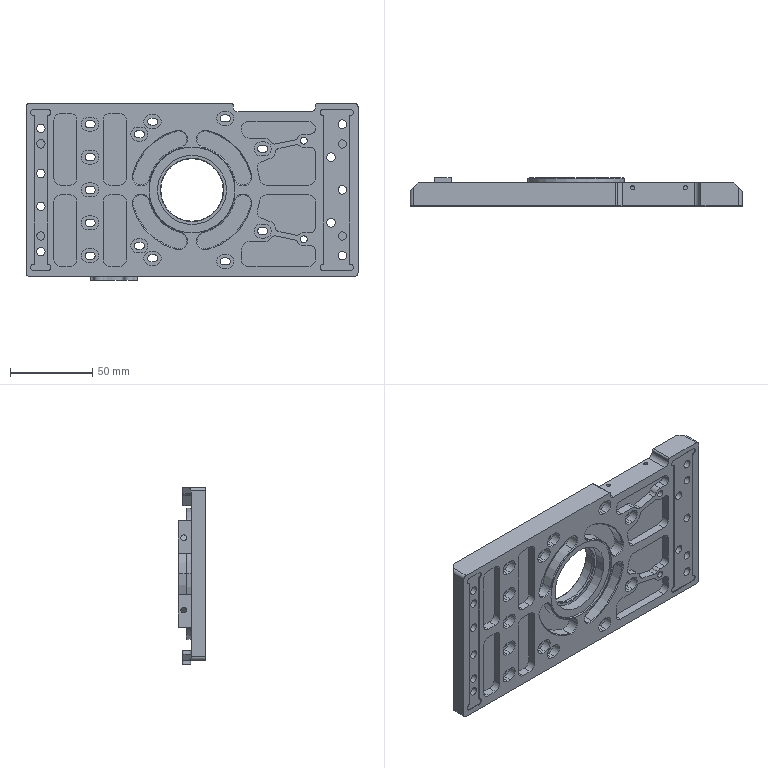CAM job | Mastercam | 3-axis milling, 5-axis milling, drilling | part box 202 x 17 x 107.5 mm | stock box 210 x 17 x 115 mm
Tools:
tool_number,name,type,diameter_mm,corner_radius_mm,flutes,flute_length_mm,overall_length_mm,shoulder_length_mm,holder_diameter_mm,length_offset,diameter_offset,default_rpm,default_feed_mm_min,default_plunge_mm_min,coolant
1,3.3 Drill,drill,3.3,0,2,25,50,40,50,1,1,1818,218.16,600,COOL_OFF
3,3 Flat End Mill,end mill,3,0,4,25,75,25,50,3,3,3333,399.96,600,COOL_OFF
4,4 Flat End Mill,end mill,4,0,4,25,75,25,50,4,4,2500,300,600,COOL_OFF
5,5 Flat End Mill,end mill,5,0,4,25,75,25,50,5,5,2000,240,600,COOL_OFF
6,6 Flat End Mill,end mill,6,0,4,25,75,25,50,6,6,1667,200.04,600,COOL_OFF
7,4 Chamfer Mill,chamfer mill,4,0,4,25,75,30,50,7,7,6250,750,600,COOL_OFF
8,8 Flat End Mill,end mill,8,0,4,25,75,25,50,8,8,1250,150,600,COOL_OFF
9,8 Bull Nose Mill,bull end mill,8,1,4,25,100,25,50,9,9,1500,180,600,COOL_OFF
10,10 Flat End Mill,end mill,10,0,4,25,75,25,50,10,10,1000,120,600,COOL_OFF
11,10 Flat End Mill,end mill,10,0,4,25,75,25,50,11,11,1000,120,600,COOL_OFF
15,4 Ball Mill / Bull Nose Mill,ball end mill,4,2,4,25,100,30,50,15,15,3000,360,600,COOL_OFF
16,16 Flat End Mill,end mill,16,0,4,25,75,25,50,16,16,2000,1000,600,COOL_OFF
16,16 Flat End Mill,end mill,16,0,4,25,75,25,50,16,16,2000,1000,600,COOL_OFF
20,63 Flat End Mill,end mill,63,0,4,25,75,25,50,20,20,159,19.08,600,COOL_OFF
24,100 Flat End Mill,end mill,100,0,4,25,75,25,50,24,24,4000,1000,600,COOL_OFF
Operations:
seq,operation,operation_type,tool_number,tool_name,tool_diameter_mm,spindle_rpm,feed_mm_min,plunge_mm_min,retract_mm_min,cycle_time_s,wcs,posted,nc_file
1,Facing - [WCS: Plane] - [Tplane: Frt],Facing,24,100 Flat End Mill,100,4000,1000,600,1200,44.776,Plane,yes,.nc
2,2D High Speed (2D Dynamic Mill) - [WCS: Plane] - [Tplane: Frt],HighSpeed2D,10,10 Flat End Mill,10,8000,3000,600,1200,115.402,Plane,yes,.nc
3,3D High Speed (Dynamic OptiRough) - [WCS: Plane] - [Tplane: Frt],HighSpeed3D,10,10 Flat End Mill,10,8000,3000,600,1200,147.199,Plane,yes,.nc
4,Contour (Remachining) - [WCS: Plane] - [Tplane: Frt],Contour,6,6 Flat End Mill,6,6500,3000,600,1200,18.374,Plane,yes,.nc
5,Contour (Remachining) - [WCS: Plane] - [Tplane: Frt],Contour,6,6 Flat End Mill,6,6500,1000,600,1200,10.217,Plane,yes,.nc
6,2D High Speed (2D Area Mill) - [WCS: Plane] - [Tplane: Frt],HighSpeed2D,6,6 Flat End Mill,6,10000,4000,600,1200,273.563,Plane,yes,.nc
7,Contour (2D) - [WCS: Plane] - [Tplane: Frt],Contour,6,6 Flat End Mill,6,10000,1000,600,1200,26.272,Plane,yes,.nc
8,Contour (2D) - [WCS: Plane] - [Tplane: Frt],Contour,11,10 Flat End Mill,10,6000,1000,600,1200,41.925,Plane,yes,.nc
9,Contour (2D) - [WCS: Plane] - [Tplane: Frt],Contour,11,10 Flat End Mill,10,6000,1000,600,1200,6.727,Plane,yes,.nc
10,Manual Entry (To),ManualEntry,,,,0,0,0,0,0,Plane-3,yes,.nc
11,Contour (2D) - [WCS: Plane] - [Tplane: Frt],Contour,11,10 Flat End Mill,10,6000,1000,600,1200,7.44,Plane,yes,.nc
12,Contour (2D) - [WCS: Plane] - [Tplane: Frt],Contour,11,10 Flat End Mill,10,6000,1000,600,1200,9.314,Plane,yes,.nc
13,Contour (Ramp) - [WCS: Plane] - [Tplane: Frt],Contour,8,8 Flat End Mill,8,10000,4000,600,1200,57.792,Plane,yes,.nc
14,Contour (2D) - [WCS: Plane] - [Tplane: Frt],Contour,8,8 Flat End Mill,8,10000,1000,600,1200,25.334,Plane,yes,.nc
15,Contour (Ramp) - [WCS: Plane] - [Tplane: Frt],Contour,8,8 Flat End Mill,8,10000,4000,600,1200,6.01,Plane,yes,.nc
16,Contour (Ramp) - [WCS: Plane] - [Tplane: Frt],Contour,5,5 Flat End Mill,5,10000,4000,600,1200,95.643,Plane,yes,.nc
17,Contour (Ramp) - [WCS: Plane] - [Tplane: Frt],Contour,5,5 Flat End Mill,5,10000,1000,600,1200,97.456,Plane,yes,.nc
18,Contour (Ramp) - [WCS: Plane] - [Tplane: Frt],Contour,5,5 Flat End Mill,5,10000,3000,600,1200,8.87,Plane,yes,.nc
19,Contour (Ramp) - [WCS: Plane] - [Tplane: Frt],Contour,5,5 Flat End Mill,5,8000,3000,600,1200,77.021,Plane,yes,.nc
20,Contour (2D) - [WCS: Plane] - [Tplane: Frt],Contour,4,4 Flat End Mill,4,8000,800,600,1200,40.742,Plane,yes,.nc
21,Contour (Remachining) - [WCS: Plane] - [Tplane: Frt],Contour,3,3 Flat End Mill,3,7000,3000,600,1200,4.935,Plane,yes,.nc
22,2D High Speed (2D Area Mill) - [WCS: Plane] - [Tplane: Frt],HighSpeed2D,3,3 Flat End Mill,3,7000,1000,600,1200,82.469,Plane,yes,.nc
23,Contour (2D) - [WCS: Plane] - [Tplane: Frt],Contour,3,3 Flat End Mill,3,7003,1000,600,1200,14.958,Plane,yes,.nc
24,Contour (Remachining) - [WCS: Plane] - [Tplane: Frt],Contour,3,3 Flat End Mill,3,7000,3000,600,1200,5.367,Plane,yes,.nc
25,Contour (2D) - [WCS: Plane] - [Tplane: Frt],Contour,3,3 Flat End Mill,3,7000,1000,600,1200,25.434,Plane,yes,.nc
26,Contour (Ramp) - [WCS: Plane] - [Tplane: Frt],Contour,3,3 Flat End Mill,3,7000,2000,600,1200,89.778,Plane,yes,.nc
27,Contour (Ramp) - [WCS: Plane] - [Tplane: Frt],Contour,3,3 Flat End Mill,3,7000,800,600,1200,37.35,Plane,yes,.nc
28,Drill/Counterbore - [WCS: Plane] - [Tplane: Frt],Drill,7,4 Chamfer Mill,4,6000,200,600,1200,15.719,Plane,yes,.nc
29,Contour (2D chamfer) - [WCS: Plane] - [Tplane: Frt],Contour,7,4 Chamfer Mill,4,7000,1000,600,1200,179.932,Plane,yes,.nc
30,Contour (2D chamfer) - [WCS: Plane] - [Tplane: Frt],Contour,7,4 Chamfer Mill,4,6000,1000,600,1200,36.133,Plane,yes,.nc
31,Contour (2D chamfer) - [WCS: Plane] - [Tplane: Frt],Contour,7,4 Chamfer Mill,4,6000,1000,600,1200,29.779,Plane,yes,.nc
32,Facing - [WCS: Plane-1] - [Tplane: Plane-1],Facing,24,100 Flat End Mill,100,4000,2000,600,1200,184.828,Plane-1,yes,.nc
33,2D High Speed (2D Area Mill) - [WCS: Plane-1] - [Tplane: Plane-1],HighSpeed2D,8,8 Flat End Mill,8,8000,4000,600,1200,1155.643,Plane-1,yes,.nc
34,Contour (2D) - [WCS: Plane-1] - [Tplane: Plane-1],Contour,8,8 Flat End Mill,8,6500,1000,600,1200,21.738,Plane-1,yes,.nc
35,Facing - [WCS: Plane-1] - [Tplane: Plane-1],Facing,8,8 Flat End Mill,8,6500,1000,600,1200,12.834,Plane-1,yes,.nc
36,Contour (2D) - [WCS: Plane-1] - [Tplane: Plane-1],Contour,8,8 Flat End Mill,8,6000,1000,600,1200,30.466,Plane-1,yes,.nc
37,Manual Entry (To),ManualEntry,,,,0,0,0,0,0,Plane-1,yes,.nc
38,Contour (2D) - [WCS: Plane-1] - [Tplane: Plane-1],Contour,8,8 Flat End Mill,8,6000,1000,600,1200,28.293,Plane-1,yes,.nc
39,Contour (Ramp) - [WCS: Plane-1] - [Tplane: Plane-1],Contour,10,10 Flat End Mill,10,10000,4000,600,1200,35.222,Plane-1,yes,.nc
40,Contour (Ramp) - [WCS: Plane-1] - [Tplane: Plane-1],Contour,10,10 Flat End Mill,10,10000,4000,600,1200,51.075,Plane-1,yes,.nc
41,Contour (Ramp) - [WCS: Plane-1] - [Tplane: Plane-1],Contour,10,10 Flat End Mill,10,10000,4000,600,1200,15.94,Plane-1,yes,.nc
42,Contour (2D) - [WCS: Plane-1] - [Tplane: Plane-1],Contour,11,10 Flat End Mill,10,10000,1000,600,1200,28.189,Plane-1,yes,.nc
43,Contour (2D) - [WCS: Plane-1] - [Tplane: Plane-1],Contour,11,10 Flat End Mill,10,6000,1000,600,1200,29.15,Plane-1,yes,.nc
44,Surface Finish Flowline - [WCS: Plane-1] - [Tplane: Plane-1],MultiSurfaceFinishFlowline,9,8 Bull Nose Mill,8,8000,4000,600,1200,37.685,Plane-1,yes,.nc
45,Contour (Remachining) - [WCS: Plane-1] - [Tplane: Plane-1],Contour,3,3 Flat End Mill,3,6000,2000,600,1200,8.849,Plane-1,yes,.nc
46,Surface Finish Flowline - [WCS: Plane-1] - [Tplane: Plane-1],MultiSurfaceFinishFlowline,15,4 Ball Mill / Bull Nose Mill,4,8000,2500,600,1200,74.406,Plane-1,yes,.nc
47,Deburr 5-axis - [WCS: Plane-1] - [Tplane: Plane-1],459,15,4 Ball Mill / Bull Nose Mill,4,6500,1000,600,1200,126.059,Plane-1,yes,.nc
48,Contour (2D chamfer) - [WCS: Plane-1] - [Tplane: Plane-1],Contour,7,4 Chamfer Mill,4,6500,1000,600,1200,46.681,Plane-1,yes,.nc
49,Manual Entry (To),ManualEntry,,,,0,0,0,0,0,Plane-1,yes,.nc
50,Contour (2D) - [WCS: Plane-1] - [Tplane: Plane-1],Contour,11,10 Flat End Mill,10,6000,1000,600,1200,7.434,Plane-1,yes,.nc
51,Drill/Counterbore - [WCS: Plane-2] - [Tplane: Plane-2],Drill,7,4 Chamfer Mill,4,6000,200,600,1200,2.184,Plane-2,yes,.nc
52,Drill/Counterbore - [WCS: Plane-3] - [Tplane: Plane-3],Drill,7,4 Chamfer Mill,4,3000,200,600,1200,2.376,Plane-3,yes,.nc
53,Peck Drill - [WCS: Plane-3] - [Tplane: Plane-3],Drill,1,3.3 Drill,3.3,1200,100,600,1200,17.952,Plane-3,yes,.nc
54,Chamfer Drill - [WCS: Plane-3] - [Tplane: Plane-3],ChamferDrill,7,4 Chamfer Mill,4,6000,200,600,1200,4.409,Plane-3,yes,.nc